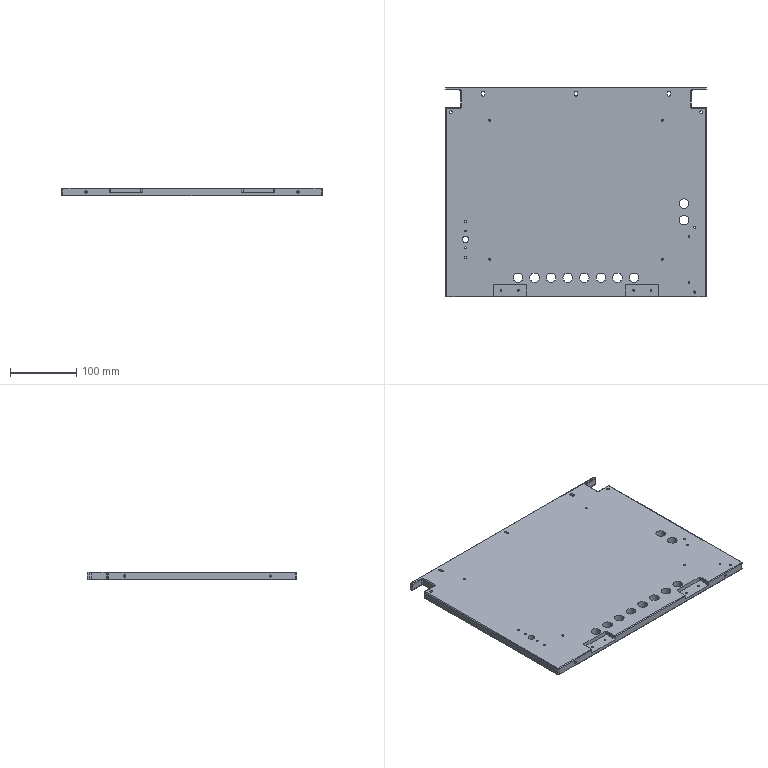CAM job | NX | 3-axis milling, drilling | part box 393.6 x 317 x 12 mm | stock box 398.6 x 322 x 12 mm
Tools:
number,name,description,diameter,corner_radius,flute_length,length,flutes
3,D3,平底铣刀-粗,3.0,0.0,20.0,75.0,2
6,D6,平底铣刀-粗,6.0,0.0,25.0,75.0,2
8,D8,平底铣刀-粗,8.0,0.0,30.0,75.0,2
9,D10,平底铣刀-粗,10.0,0.0,35.0,75.0,2
11,D3-J,平底铣刀-精,3.0,0.0,50.0,75.0,2
7,D6-J,平底铣刀-精,6.0,0.0,25.0,75.0,2
10,D10-J,平底铣刀-精,10.0,0.0,35.0,75.0,2
17,D4R0.5,圆鼻刀-粗,4.0,0.5,50.0,75.0,2
2,D6倒角刀,倒角刀,6.0,0.0,3.0,25.0,2
20,M3X0.5,丝锥,2.5,0.0,35.0,50.0,2
21,M4X0.7,丝锥,3.3,0.0,35.0,50.0,2
22,M5X0.8,丝锥,4.2,0.0,35.0,50.0,2
12,ZT2.5,钻头,2.5,0.0,35.0,50.0,2
13,钻头3.3,Twist Drill 3.3 mm,3.3,0.0,35.0,35.008,2
14,钻头4.2,Twist Drill 4.2 mm,4.2,0.0,41.0,41.738,2
Operations:
program,operation,operation_type,tool,method,geometry_group,spindle_rpm,surface_speed,feed_per_tooth,feed_cut,feed_plunge,cut_length_mm,path_length_mm,cut_time_min,machine_time_min
B,底壁铣分层开粗-中_COPY,VolumeBased25DMillingOperation,D10,分层开粗-切深K-步距G,W-B,8000.0,251.32,0.25,4000.0,100.0,3613.887,4368.769,0.9035,0.979
B,打点-深0.8,Operation,D6倒角刀,NONE,W-B,8000.0,150.796,0.0312,500.0,90.0,52.2,1240.66,0.1044,0.2232
B,通孔-M3螺纹底孔,Operation,ZT2.5,NONE,W-B,3000.0,23.562,0.05,300.0,90.0,124.409,759.167,0.4147,0.4782
B,通孔-M4螺纹底孔,Operation,钻头3.3,NONE,W-B,3000.0,31.102,0.05,300.0,90.0,119.931,1103.251,0.3998,0.4981
B,通孔-M5螺纹底孔,Operation,钻头4.2,NONE,W-B,3000.0,39.584,0.0583,350.0,90.0,40.524,499.85,0.1158,0.1617
B,等高光顺清角D3参考8_COPY_1,ZLevelMilling,D3-J,分层精光-切深K-步距G,W-B,8000.0,75.398,0.1125,1800.0,100.0,2022.542,2370.797,1.124,1.159
B,等高精光往复爬面_COPY,ZLevelMilling,D4R0.5,等高爬面-切深K-步距G,W-B,7000.0,87.965,0.3571,5000.0,100.0,35488.084,35574.952,7.098,7.106
B,C0.3封闭铣廓倒角6X45L_COPY,PlanarMilling,D6倒角刀,爬面_倒角-切深0-步距G,W-B,7000.0,131.0,0.1071,1500.0,100.0,671.05,2091.528,0.4474,0.5894
B,钻倒角_4,Operation,D6倒角刀,METHOD,W-B,8000.0,150.796,0.0312,500.0,0.0,38.0,600.947,0.076,0.1323
B,钻倒角_5,Operation,D6倒角刀,METHOD,W-B,8000.0,150.796,0.0312,500.0,0.0,41.6,960.949,0.0832,0.1751
B,铣倒角_2,PlanarMilling,D6倒角刀,METHOD,W-B,8000.0,150.796,0.0312,500.0,100.0,36.041,496.027,0.0721,0.1181
B,铣倒角_3,PlanarMilling,D6倒角刀,METHOD,W-B,8000.0,150.796,0.0312,500.0,100.0,37.443,78.442,0.0749,0.079
B,平面去毛刺6X45L_COPY,SurfaceContour,D6倒角刀,爬面_倒角-切深0-步距G,W-B,6500.0,122.519,0.1154,1500.0,100.0,295.452,1085.431,0.197,0.276
B,通孔-攻牙M3,Operation,M3X0.5,METHOD,W-B,800.0,6.283,0.0003,0.5,90.0,128.0,765.792,256.0,256.064
B,通孔-攻牙M4,Operation,M4X0.7,METHOD,W-B,600.0,6.22,0.0006,0.7,90.0,96.0,1055.388,137.143,137.239
B,通孔-攻牙M5,Operation,M5X0.8,METHOD,W-B,500.0,6.597,0.0008,0.8,90.0,33.0,484.803,41.25,41.295
B,底壁铣精光底面-中_COPY,VolumeBased25DMillingOperation,D6-J,精光步距切深关,W-B,8000.0,150.792,0.0625,1000.0,100.0,594.232,862.003,0.5942,0.621
B,底壁铣精光侧面-中-选底面_COPY,VolumeBased25DMillingOperation,D6-J,侧刃精光-切深K-步距G,W-B,8000.0,150.792,0.0625,1000.0,100.0,176.338,456.339,0.1763,0.2043
A,底壁粗_1,VolumeBased25DMillingOperation,D10,METHOD,W-A,8000.0,251.327,0.2188,3500.0,100.0,159957.806,161865.462,45.702,45.893
A,外形粗_2,VolumeBased25DMillingOperation,D10,METHOD,W-A,6000.0,188.0,0.25,4000.0,80.0,39828.173,39878.173,9.957,9.962
A,盲腰槽粗,VolumeBased25DMillingOperation,D6,METHOD,W-A,8000.0,150.796,0.075,1200.0,100.0,1018.612,1429.114,0.8488,0.8899
A,底壁铣螺旋开粗-中_COPY_COPY,VolumeBased25DMillingOperation,D6,分层开粗-切深K-步距G,W-A,8000.0,150.796,0.125,2000.0,100.0,510.113,559.913,0.2551,0.26
A,底壁铣螺旋开粗-中_COPY,VolumeBased25DMillingOperation,D8,分层开粗-切深K-步距G,W-A,8000.0,150.796,0.125,2000.0,100.0,8320.687,9285.849,4.16,4.257
A,通腰槽粗_1,VolumeBased25DMillingOperation,D3,METHOD,W-A,6000.0,75.398,0.1,1200.0,100.0,942.583,1387.185,0.7855,0.8299
A,等高光顺清角D3参考8_COPY,ZLevelMilling,D3-J,分层精光-切深K-步距G,W-A,8000.0,75.396,0.05,800.0,100.0,3731.287,4258.322,4.664,4.717
A,等高螺旋爬面_COPY,ZLevelMilling,D4R0.5,等高爬面-切深K-步距G,W-A,7000.0,175.924,0.1786,2500.0,100.0,34872.566,34911.066,13.949,13.953
A,仅选体,SurfaceContour,D6倒角刀,METHOD,W-A,6000.0,113.0,0.125,1200.0,100.0,1622.665,3121.46,1.352,1.502
A,钻倒角_1,Operation,D6倒角刀,METHOD,W-A,5000.0,94.248,0.015,150.0,0.0,38.0,600.454,0.2533,0.3096
A,钻倒角_2,Operation,D6倒角刀,METHOD,W-A,5000.0,94.248,0.015,150.0,0.0,41.6,970.489,0.2773,0.3702
A,钻倒角_3,Operation,D6倒角刀,METHOD,W-A,5000.0,94.248,0.015,150.0,0.0,11.4,443.613,0.076,0.1192
A,铣倒角_1,PlanarMilling,D6倒角刀,METHOD,W-A,6000.0,113.097,0.05,600.0,100.0,37.443,78.442,0.0624,0.0665
A,腰槽精,VolumeBased25DMillingOperation,D6-J,METHOD,W-A,6000.0,113.0,0.0667,300.0,100.0,87.069,530.273,0.2902,0.3346
A,底壁铣精光侧面-中_COPY,VolumeBased25DMillingOperation,D6-J,侧刃精光-切深K-步距G,W-A,8000.0,150.792,0.0625,1000.0,100.0,355.902,1523.11,0.3559,0.4726
A,腰槽精_3,VolumeBased25DMillingOperation,D3-J,METHOD,W-A,6000.0,113.0,0.0417,500.0,100.0,77.644,570.548,0.1553,0.2046
A,底精_1,VolumeBased25DMillingOperation,D10-J,METHOD,W-A,6000.0,113.0,0.2083,1200.0,100.0,9981.181,10035.181,8.318,8.323
A,底侧精_3,VolumeBased25DMillingOperation,D10-J,METHOD,W-A,6000.0,113.0,0.2083,1200.0,100.0,1032.842,1087.832,0.8607,0.8662
A,外形半精_2,VolumeBased25DMillingOperation,D6-J,METHOD,W-A,6000.0,113.0,0.0833,1000.0,100.0,1527.147,1589.147,1.527,1.533
A,外形精_2,VolumeBased25DMillingOperation,D6-J,METHOD,W-A,6000.0,113.0,0.0833,1000.0,100.0,1526.947,1589.547,1.527,1.533